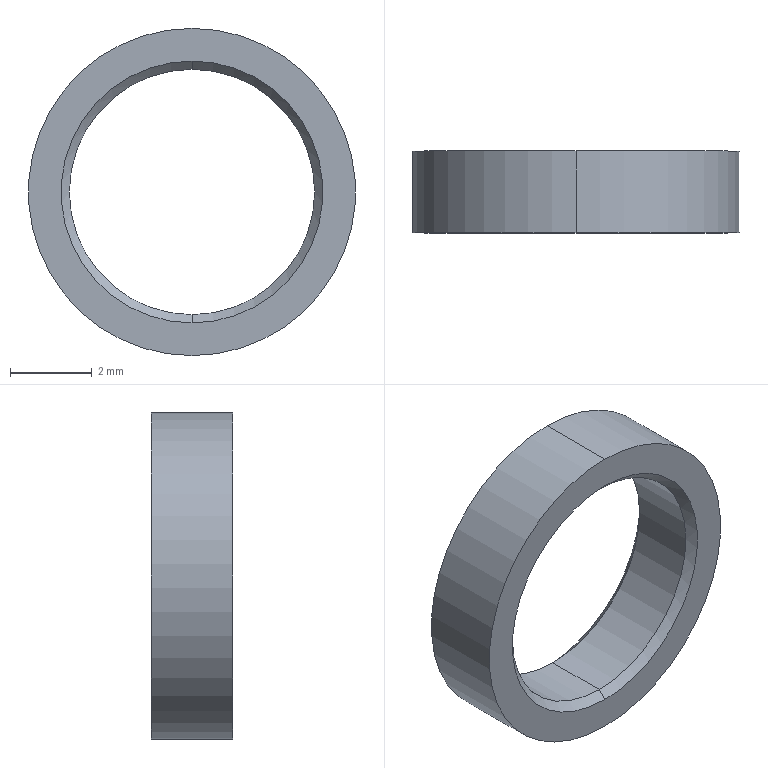Part | SolidWorks | features Chamfer 1, Extrusion 1 | 1 solid | 10 faces | box 8 x 2 x 8 mm | volume 43.212 mm3 | cone 4 | cylinder 4 | plane 2 | commonest cylinder face diameters 6 x2 8 x2
STEP:
#1=CARTESIAN_POINT('',(0.,1.8,-3.));
#2=VERTEX_POINT('',#1);
#3=CARTESIAN_POINT('',(0.,1.8,3.));
#4=VERTEX_POINT('',#3);
#5=CARTESIAN_POINT('',(0.,1.8,0.));
#6=DIRECTION('',(0.,1.,0.));
#7=DIRECTION('',(0.,0.,1.));
#8=AXIS2_PLACEMENT_3D('',#5,#6,#7);
#9=CIRCLE('',#8,3.);
#10=EDGE_CURVE('',#2,#4,#9,.T.);
#11=ORIENTED_EDGE('',*,*,#10,.F.);
#12=CARTESIAN_POINT('',(0.,2.,-3.2));
#13=VERTEX_POINT('',#12);
#14=CARTESIAN_POINT('',(0.,1.8,-3.));
#15=DIRECTION('',(0.,0.7071,-0.7071));
#16=VECTOR('',#15,1000.);
#17=LINE('',#14,#16);
#18=EDGE_CURVE('',#2,#13,#17,.T.);
#19=ORIENTED_EDGE('',*,*,#18,.T.);
#20=CARTESIAN_POINT('',(0.,2.,3.2));
#21=VERTEX_POINT('',#20);
#22=CARTESIAN_POINT('',(0.,2.,0.));
#23=DIRECTION('',(0.,-1.,0.));
#24=DIRECTION('',(0.,0.,1.));
#25=AXIS2_PLACEMENT_3D('',#22,#23,#24);
#26=CIRCLE('',#25,3.2);
#27=EDGE_CURVE('',#21,#13,#26,.T.);
#28=ORIENTED_EDGE('',*,*,#27,.F.);
#29=CARTESIAN_POINT('',(0.,1.8,3.));
#30=DIRECTION('',(0.,0.7071,0.7071));
#31=VECTOR('',#30,1000.);
#32=LINE('',#29,#31);
#33=EDGE_CURVE('',#4,#21,#32,.T.);
#34=ORIENTED_EDGE('',*,*,#33,.F.);
#35=EDGE_LOOP('',(#11,#19,#28,#34));
#36=FACE_OUTER_BOUND('',#35,.T.);
#37=CARTESIAN_POINT('',(0.,1.8,0.));
#38=DIRECTION('',(0.,1.,0.));
#39=DIRECTION('',(0.,0.,1.));
#40=AXIS2_PLACEMENT_3D('',#37,#38,#39);
#41=CONICAL_SURFACE('',#40,3.,0.7854);
#42=ADVANCED_FACE('',(#36),#41,.F.);
#43=CARTESIAN_POINT('',(0.,0.2,3.));
#44=VERTEX_POINT('',#43);
#45=CARTESIAN_POINT('',(0.,0.2,-3.));
#46=VERTEX_POINT('',#45);
#47=CARTESIAN_POINT('',(0.,0.2,0.));
#48=DIRECTION('',(0.,-1.,0.));
#49=DIRECTION('',(0.,0.,1.));
#50=AXIS2_PLACEMENT_3D('',#47,#48,#49);
#51=CIRCLE('',#50,3.);
#52=EDGE_CURVE('',#44,#46,#51,.T.);
#53=ORIENTED_EDGE('',*,*,#52,.F.);
#54=CARTESIAN_POINT('',(0.,0.,3.2));
#55=VERTEX_POINT('',#54);
#56=CARTESIAN_POINT('',(0.,0.,3.2));
#57=DIRECTION('',(0.,-0.7071,0.7071));
#58=VECTOR('',#57,1000.);
#59=LINE('',#56,#58);
#60=EDGE_CURVE('',#44,#55,#59,.T.);
#61=ORIENTED_EDGE('',*,*,#60,.T.);
#62=CARTESIAN_POINT('',(0.,0.,-3.2));
#63=VERTEX_POINT('',#62);
#64=CARTESIAN_POINT('',(0.,0.,0.));
#65=DIRECTION('',(0.,1.,0.));
#66=DIRECTION('',(0.,0.,1.));
#67=AXIS2_PLACEMENT_3D('',#64,#65,#66);
#68=CIRCLE('',#67,3.2);
#69=EDGE_CURVE('',#63,#55,#68,.T.);
#70=ORIENTED_EDGE('',*,*,#69,.F.);
#71=CARTESIAN_POINT('',(0.,0.,-3.2));
#72=DIRECTION('',(0.,-0.7071,-0.7071));
#73=VECTOR('',#72,1000.);
#74=LINE('',#71,#73);
#75=EDGE_CURVE('',#46,#63,#74,.T.);
#76=ORIENTED_EDGE('',*,*,#75,.F.);
#77=EDGE_LOOP('',(#53,#61,#70,#76));
#78=FACE_OUTER_BOUND('',#77,.T.);
#79=CARTESIAN_POINT('',(0.,0.,0.));
#80=DIRECTION('',(0.,-1.,0.));
#81=DIRECTION('',(0.,0.,-1.));
#82=AXIS2_PLACEMENT_3D('',#79,#80,#81);
#83=CONICAL_SURFACE('',#82,3.2,0.7854);
#84=ADVANCED_FACE('',(#78),#83,.F.);
#85=ORIENTED_EDGE('',*,*,#10,.T.);
#86=CARTESIAN_POINT('',(0.,2.,3.));
#87=DIRECTION('',(0.,-1.,0.));
#88=VECTOR('',#87,1000.);
#89=LINE('',#86,#88);
#90=EDGE_CURVE('',#4,#44,#89,.T.);
#91=ORIENTED_EDGE('',*,*,#90,.T.);
#92=ORIENTED_EDGE('',*,*,#52,.T.);
#93=CARTESIAN_POINT('',(0.,2.,-3.));
#94=DIRECTION('',(0.,-1.,0.));
#95=VECTOR('',#94,1000.);
#96=LINE('',#93,#95);
#97=EDGE_CURVE('',#2,#46,#96,.T.);
#98=ORIENTED_EDGE('',*,*,#97,.F.);
#99=EDGE_LOOP('',(#85,#91,#92,#98));
#100=FACE_OUTER_BOUND('',#99,.T.);
#101=CARTESIAN_POINT('',(0.,2.,0.));
#102=DIRECTION('',(0.,-1.,0.));
#103=DIRECTION('',(0.,0.,-1.));
#104=AXIS2_PLACEMENT_3D('',#101,#102,#103);
#105=CYLINDRICAL_SURFACE('',#104,3.);
#106=ADVANCED_FACE('',(#100),#105,.F.);
#107=CARTESIAN_POINT('',(0.,2.,4.));
#108=VERTEX_POINT('',#107);
#109=CARTESIAN_POINT('',(0.,2.,-4.));
#110=VERTEX_POINT('',#109);
#111=CARTESIAN_POINT('',(0.,2.,0.));
#112=DIRECTION('',(0.,1.,0.));
#113=DIRECTION('',(0.,0.,1.));
#114=AXIS2_PLACEMENT_3D('',#111,#112,#113);
#115=CIRCLE('',#114,4.);
#116=EDGE_CURVE('',#108,#110,#115,.T.);
#117=ORIENTED_EDGE('',*,*,#116,.F.);
#118=CARTESIAN_POINT('',(0.,0.,4.));
#119=VERTEX_POINT('',#118);
#120=CARTESIAN_POINT('',(0.,2.,4.));
#121=DIRECTION('',(0.,-1.,0.));
#122=VECTOR('',#121,1000.);
#123=LINE('',#120,#122);
#124=EDGE_CURVE('',#108,#119,#123,.T.);
#125=ORIENTED_EDGE('',*,*,#124,.T.);
#126=CARTESIAN_POINT('',(0.,0.,-4.));
#127=VERTEX_POINT('',#126);
#128=CARTESIAN_POINT('',(0.,0.,0.));
#129=DIRECTION('',(0.,1.,0.));
#130=DIRECTION('',(0.,0.,1.));
#131=AXIS2_PLACEMENT_3D('',#128,#129,#130);
#132=CIRCLE('',#131,4.);
#133=EDGE_CURVE('',#119,#127,#132,.T.);
#134=ORIENTED_EDGE('',*,*,#133,.T.);
#135=CARTESIAN_POINT('',(0.,2.,-4.));
#136=DIRECTION('',(0.,-1.,0.));
#137=VECTOR('',#136,1000.);
#138=LINE('',#135,#137);
#139=EDGE_CURVE('',#110,#127,#138,.T.);
#140=ORIENTED_EDGE('',*,*,#139,.F.);
#141=EDGE_LOOP('',(#117,#125,#134,#140));
#142=FACE_OUTER_BOUND('',#141,.T.);
#143=CARTESIAN_POINT('',(0.,2.,0.));
#144=DIRECTION('',(0.,-1.,0.));
#145=DIRECTION('',(0.,0.,-1.));
#146=AXIS2_PLACEMENT_3D('',#143,#144,#145);
#147=CYLINDRICAL_SURFACE('',#146,4.);
#148=ADVANCED_FACE('',(#142),#147,.T.);
#149=ORIENTED_EDGE('',*,*,#27,.T.);
#150=CARTESIAN_POINT('',(0.,2.,0.));
#151=DIRECTION('',(0.,-1.,0.));
#152=DIRECTION('',(0.,0.,1.));
#153=AXIS2_PLACEMENT_3D('',#150,#151,#152);
#154=CIRCLE('',#153,3.2);
#155=EDGE_CURVE('',#13,#21,#154,.T.);
#156=ORIENTED_EDGE('',*,*,#155,.T.);
#157=EDGE_LOOP('',(#149,#156));
#158=FACE_BOUND('',#157,.T.);
#159=CARTESIAN_POINT('',(0.,2.,0.));
#160=DIRECTION('',(0.,1.,0.));
#161=DIRECTION('',(0.,0.,1.));
#162=AXIS2_PLACEMENT_3D('',#159,#160,#161);
#163=CIRCLE('',#162,4.);
#164=EDGE_CURVE('',#110,#108,#163,.T.);
#165=ORIENTED_EDGE('',*,*,#164,.T.);
#166=ORIENTED_EDGE('',*,*,#116,.T.);
#167=EDGE_LOOP('',(#165,#166));
#168=FACE_OUTER_BOUND('',#167,.T.);
#169=CARTESIAN_POINT('',(0.,2.,0.));
#170=DIRECTION('',(0.,1.,0.));
#171=DIRECTION('',(0.,0.,1.));
#172=AXIS2_PLACEMENT_3D('',#169,#170,#171);
#173=PLANE('',#172);
#174=ADVANCED_FACE('',(#158,#168),#173,.T.);
#175=ORIENTED_EDGE('',*,*,#69,.T.);
#176=CARTESIAN_POINT('',(0.,0.,0.));
#177=DIRECTION('',(0.,1.,0.));
#178=DIRECTION('',(0.,0.,1.));
#179=AXIS2_PLACEMENT_3D('',#176,#177,#178);
#180=CIRCLE('',#179,3.2);
#181=EDGE_CURVE('',#55,#63,#180,.T.);
#182=ORIENTED_EDGE('',*,*,#181,.T.);
#183=EDGE_LOOP('',(#175,#182));
#184=FACE_BOUND('',#183,.T.);
#185=CARTESIAN_POINT('',(0.,0.,0.));
#186=DIRECTION('',(0.,1.,0.));
#187=DIRECTION('',(0.,0.,1.));
#188=AXIS2_PLACEMENT_3D('',#185,#186,#187);
#189=CIRCLE('',#188,4.);
#190=EDGE_CURVE('',#127,#119,#189,.T.);
#191=ORIENTED_EDGE('',*,*,#190,.F.);
#192=ORIENTED_EDGE('',*,*,#133,.F.);
#193=EDGE_LOOP('',(#191,#192));
#194=FACE_OUTER_BOUND('',#193,.T.);
#195=CARTESIAN_POINT('',(0.,0.,0.));
#196=DIRECTION('',(0.,1.,0.));
#197=DIRECTION('',(0.,0.,1.));
#198=AXIS2_PLACEMENT_3D('',#195,#196,#197);
#199=PLANE('',#198);
#200=ADVANCED_FACE('',(#184,#194),#199,.F.);
#201=ORIENTED_EDGE('',*,*,#124,.F.);
#202=ORIENTED_EDGE('',*,*,#164,.F.);
#203=ORIENTED_EDGE('',*,*,#139,.T.);
#204=ORIENTED_EDGE('',*,*,#190,.T.);
#205=EDGE_LOOP('',(#201,#202,#203,#204));
#206=FACE_OUTER_BOUND('',#205,.T.);
#207=CARTESIAN_POINT('',(0.,2.,0.));
#208=DIRECTION('',(0.,-1.,0.));
#209=DIRECTION('',(0.,0.,-1.));
#210=AXIS2_PLACEMENT_3D('',#207,#208,#209);
#211=CYLINDRICAL_SURFACE('',#210,4.);
#212=ADVANCED_FACE('',(#206),#211,.T.);
#213=ORIENTED_EDGE('',*,*,#90,.F.);
#214=CARTESIAN_POINT('',(0.,1.8,0.));
#215=DIRECTION('',(0.,1.,0.));
#216=DIRECTION('',(0.,0.,1.));
#217=AXIS2_PLACEMENT_3D('',#214,#215,#216);
#218=CIRCLE('',#217,3.);
#219=EDGE_CURVE('',#4,#2,#218,.T.);
#220=ORIENTED_EDGE('',*,*,#219,.T.);
#221=ORIENTED_EDGE('',*,*,#97,.T.);
#222=CARTESIAN_POINT('',(0.,0.2,0.));
#223=DIRECTION('',(0.,-1.,0.));
#224=DIRECTION('',(0.,0.,1.));
#225=AXIS2_PLACEMENT_3D('',#222,#223,#224);
#226=CIRCLE('',#225,3.);
#227=EDGE_CURVE('',#46,#44,#226,.T.);
#228=ORIENTED_EDGE('',*,*,#227,.T.);
#229=EDGE_LOOP('',(#213,#220,#221,#228));
#230=FACE_OUTER_BOUND('',#229,.T.);
#231=CARTESIAN_POINT('',(0.,2.,0.));
#232=DIRECTION('',(0.,-1.,0.));
#233=DIRECTION('',(0.,0.,-1.));
#234=AXIS2_PLACEMENT_3D('',#231,#232,#233);
#235=CYLINDRICAL_SURFACE('',#234,3.);
#236=ADVANCED_FACE('',(#230),#235,.F.);
#237=ORIENTED_EDGE('',*,*,#60,.F.);
#238=ORIENTED_EDGE('',*,*,#227,.F.);
#239=ORIENTED_EDGE('',*,*,#75,.T.);
#240=ORIENTED_EDGE('',*,*,#181,.F.);
#241=EDGE_LOOP('',(#237,#238,#239,#240));
#242=FACE_OUTER_BOUND('',#241,.T.);
#243=CARTESIAN_POINT('',(0.,0.,0.));
#244=DIRECTION('',(0.,-1.,0.));
#245=DIRECTION('',(0.,0.,-1.));
#246=AXIS2_PLACEMENT_3D('',#243,#244,#245);
#247=CONICAL_SURFACE('',#246,3.2,0.7854);
#248=ADVANCED_FACE('',(#242),#247,.F.);
#249=ORIENTED_EDGE('',*,*,#18,.F.);
#250=ORIENTED_EDGE('',*,*,#219,.F.);
#251=ORIENTED_EDGE('',*,*,#33,.T.);
#252=ORIENTED_EDGE('',*,*,#155,.F.);
#253=EDGE_LOOP('',(#249,#250,#251,#252));
#254=FACE_OUTER_BOUND('',#253,.T.);
#255=CARTESIAN_POINT('',(0.,1.8,0.));
#256=DIRECTION('',(0.,1.,0.));
#257=DIRECTION('',(0.,0.,1.));
#258=AXIS2_PLACEMENT_3D('',#255,#256,#257);
#259=CONICAL_SURFACE('',#258,3.,0.7854);
#260=ADVANCED_FACE('',(#254),#259,.F.);
#261=CLOSED_SHELL('',(#42,#84,#106,#148,#174,#200,#212,#236,#248,#260));
#262=MANIFOLD_SOLID_BREP('',#261);
#263=CARTESIAN_POINT('',(0.,0.,0.));
#264=DIRECTION('',(0.,0.,1.));
#265=DIRECTION('',(1.,0.,0.));
#266=AXIS2_PLACEMENT_3D('',#263,#264,#265);
#267=(LENGTH_UNIT()NAMED_UNIT(*)SI_UNIT(.MILLI.,.METRE.));
#268=UNCERTAINTY_MEASURE_WITH_UNIT(LENGTH_MEASURE(0.00001),#267,'','');
#269=(NAMED_UNIT(*)PLANE_ANGLE_UNIT()SI_UNIT($,.RADIAN.));
#270=(NAMED_UNIT(*)SI_UNIT($,.STERADIAN.)SOLID_ANGLE_UNIT());
#271=(GEOMETRIC_REPRESENTATION_CONTEXT(3)GLOBAL_UNCERTAINTY_ASSIGNED_CONTEXT((#268))GLOBAL_UNIT_ASSIGNED_CONTEXT((#267,#269,#270))REPRESENTATION_CONTEXT('',''));
#272=ADVANCED_BREP_SHAPE_REPRESENTATION('',(#262,#266),#271);